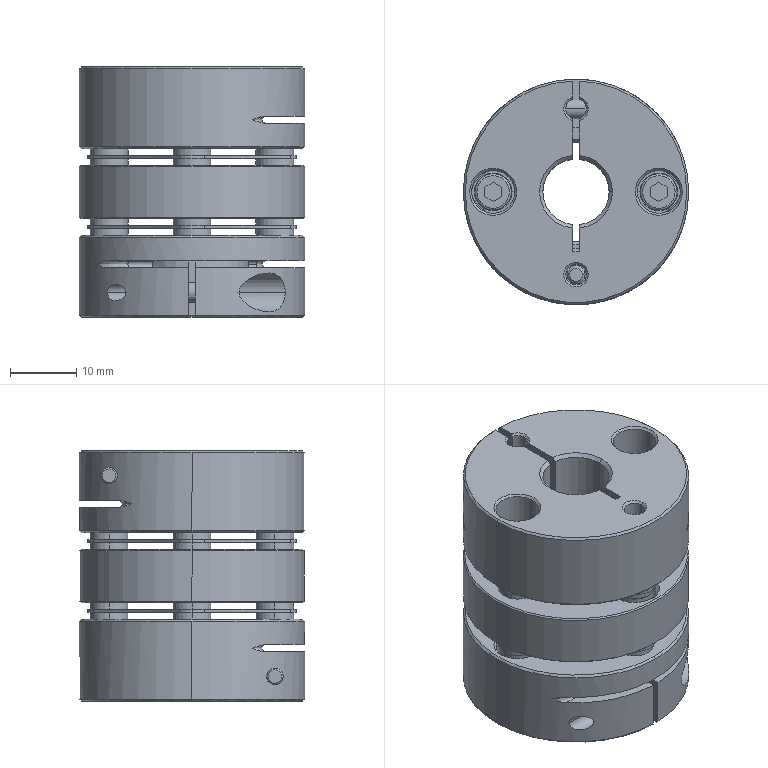Part | STEP file | double-diaphragm coupling LC-A-030DA-10B-10B | 1 solid | 435 faces | box 34 x 34 x 37.8 mm | volume 23948 mm3 | cylinder 176 | plane 149 | cone 104 | spline 6 | commonest cylinder face diameters 5.7 x32 5.5 x20 3.1 x16 6.5 x16 2.75 x12 3 x12